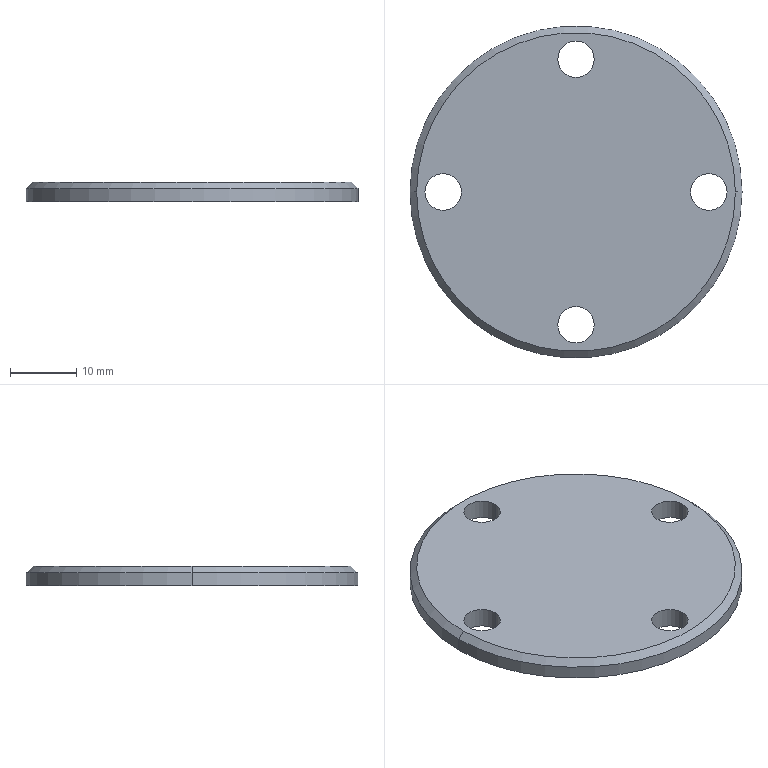Part | SolidWorks | features Chamfer 1, Extrusion 1, ICE 1 | 1 solid | 14 faces | box 50 x 50 x 3 mm | volume 5528 mm3 | cylinder 10 | cone 2 | plane 2 | commonest cylinder face diameters 5.5 x8 50 x2
STEP:
#1=CARTESIAN_POINT('',(17.25,0.,0.));
#2=VERTEX_POINT('',#1);
#3=CARTESIAN_POINT('',(22.75,0.,0.));
#4=VERTEX_POINT('',#3);
#5=CARTESIAN_POINT('',(20.,0.,0.));
#6=DIRECTION('',(0.,0.,1.));
#7=DIRECTION('',(1.,0.,0.));
#8=AXIS2_PLACEMENT_3D('',#5,#6,#7);
#9=CIRCLE('',#8,2.75);
#10=EDGE_CURVE('',#2,#4,#9,.T.);
#11=ORIENTED_EDGE('',*,*,#10,.F.);
#12=CARTESIAN_POINT('',(17.25,0.,3.));
#13=VERTEX_POINT('',#12);
#14=CARTESIAN_POINT('',(17.25,0.,0.));
#15=DIRECTION('',(0.,0.,1.));
#16=VECTOR('',#15,1000.);
#17=LINE('',#14,#16);
#18=EDGE_CURVE('',#2,#13,#17,.T.);
#19=ORIENTED_EDGE('',*,*,#18,.T.);
#20=CARTESIAN_POINT('',(22.75,0.,3.));
#21=VERTEX_POINT('',#20);
#22=CARTESIAN_POINT('',(20.,0.,3.));
#23=DIRECTION('',(0.,0.,1.));
#24=DIRECTION('',(1.,0.,0.));
#25=AXIS2_PLACEMENT_3D('',#22,#23,#24);
#26=CIRCLE('',#25,2.75);
#27=EDGE_CURVE('',#13,#21,#26,.T.);
#28=ORIENTED_EDGE('',*,*,#27,.T.);
#29=CARTESIAN_POINT('',(22.75,0.,0.));
#30=DIRECTION('',(0.,0.,1.));
#31=VECTOR('',#30,1000.);
#32=LINE('',#29,#31);
#33=EDGE_CURVE('',#4,#21,#32,.T.);
#34=ORIENTED_EDGE('',*,*,#33,.F.);
#35=EDGE_LOOP('',(#11,#19,#28,#34));
#36=FACE_OUTER_BOUND('',#35,.T.);
#37=CARTESIAN_POINT('',(20.,0.,0.));
#38=DIRECTION('',(0.,0.,1.));
#39=DIRECTION('',(1.,0.,0.));
#40=AXIS2_PLACEMENT_3D('',#37,#38,#39);
#41=CYLINDRICAL_SURFACE('',#40,2.75);
#42=ADVANCED_FACE('',(#36),#41,.F.);
#43=CARTESIAN_POINT('',(-2.75,-20.,0.));
#44=VERTEX_POINT('',#43);
#45=CARTESIAN_POINT('',(2.75,-20.,0.));
#46=VERTEX_POINT('',#45);
#47=CARTESIAN_POINT('',(0.,-20.,0.));
#48=DIRECTION('',(0.,0.,1.));
#49=DIRECTION('',(1.,0.,0.));
#50=AXIS2_PLACEMENT_3D('',#47,#48,#49);
#51=CIRCLE('',#50,2.75);
#52=EDGE_CURVE('',#44,#46,#51,.T.);
#53=ORIENTED_EDGE('',*,*,#52,.F.);
#54=CARTESIAN_POINT('',(-2.75,-20.,3.));
#55=VERTEX_POINT('',#54);
#56=CARTESIAN_POINT('',(-2.75,-20.,0.));
#57=DIRECTION('',(0.,0.,1.));
#58=VECTOR('',#57,1000.);
#59=LINE('',#56,#58);
#60=EDGE_CURVE('',#44,#55,#59,.T.);
#61=ORIENTED_EDGE('',*,*,#60,.T.);
#62=CARTESIAN_POINT('',(2.75,-20.,3.));
#63=VERTEX_POINT('',#62);
#64=CARTESIAN_POINT('',(0.,-20.,3.));
#65=DIRECTION('',(0.,0.,1.));
#66=DIRECTION('',(1.,0.,0.));
#67=AXIS2_PLACEMENT_3D('',#64,#65,#66);
#68=CIRCLE('',#67,2.75);
#69=EDGE_CURVE('',#55,#63,#68,.T.);
#70=ORIENTED_EDGE('',*,*,#69,.T.);
#71=CARTESIAN_POINT('',(2.75,-20.,0.));
#72=DIRECTION('',(0.,0.,1.));
#73=VECTOR('',#72,1000.);
#74=LINE('',#71,#73);
#75=EDGE_CURVE('',#46,#63,#74,.T.);
#76=ORIENTED_EDGE('',*,*,#75,.F.);
#77=EDGE_LOOP('',(#53,#61,#70,#76));
#78=FACE_OUTER_BOUND('',#77,.T.);
#79=CARTESIAN_POINT('',(0.,-20.,0.));
#80=DIRECTION('',(0.,0.,1.));
#81=DIRECTION('',(1.,0.,0.));
#82=AXIS2_PLACEMENT_3D('',#79,#80,#81);
#83=CYLINDRICAL_SURFACE('',#82,2.75);
#84=ADVANCED_FACE('',(#78),#83,.F.);
#85=CARTESIAN_POINT('',(-22.75,0.,0.));
#86=VERTEX_POINT('',#85);
#87=CARTESIAN_POINT('',(-17.25,0.,0.));
#88=VERTEX_POINT('',#87);
#89=CARTESIAN_POINT('',(-20.,0.,0.));
#90=DIRECTION('',(0.,0.,1.));
#91=DIRECTION('',(1.,0.,0.));
#92=AXIS2_PLACEMENT_3D('',#89,#90,#91);
#93=CIRCLE('',#92,2.75);
#94=EDGE_CURVE('',#86,#88,#93,.T.);
#95=ORIENTED_EDGE('',*,*,#94,.F.);
#96=CARTESIAN_POINT('',(-22.75,0.,3.));
#97=VERTEX_POINT('',#96);
#98=CARTESIAN_POINT('',(-22.75,0.,0.));
#99=DIRECTION('',(0.,0.,1.));
#100=VECTOR('',#99,1000.);
#101=LINE('',#98,#100);
#102=EDGE_CURVE('',#86,#97,#101,.T.);
#103=ORIENTED_EDGE('',*,*,#102,.T.);
#104=CARTESIAN_POINT('',(-17.25,0.,3.));
#105=VERTEX_POINT('',#104);
#106=CARTESIAN_POINT('',(-20.,0.,3.));
#107=DIRECTION('',(0.,0.,1.));
#108=DIRECTION('',(1.,0.,0.));
#109=AXIS2_PLACEMENT_3D('',#106,#107,#108);
#110=CIRCLE('',#109,2.75);
#111=EDGE_CURVE('',#97,#105,#110,.T.);
#112=ORIENTED_EDGE('',*,*,#111,.T.);
#113=CARTESIAN_POINT('',(-17.25,0.,0.));
#114=DIRECTION('',(0.,0.,1.));
#115=VECTOR('',#114,1000.);
#116=LINE('',#113,#115);
#117=EDGE_CURVE('',#88,#105,#116,.T.);
#118=ORIENTED_EDGE('',*,*,#117,.F.);
#119=EDGE_LOOP('',(#95,#103,#112,#118));
#120=FACE_OUTER_BOUND('',#119,.T.);
#121=CARTESIAN_POINT('',(-20.,0.,0.));
#122=DIRECTION('',(0.,0.,1.));
#123=DIRECTION('',(1.,0.,0.));
#124=AXIS2_PLACEMENT_3D('',#121,#122,#123);
#125=CYLINDRICAL_SURFACE('',#124,2.75);
#126=ADVANCED_FACE('',(#120),#125,.F.);
#127=CARTESIAN_POINT('',(-2.75,20.,0.));
#128=VERTEX_POINT('',#127);
#129=CARTESIAN_POINT('',(2.75,20.,0.));
#130=VERTEX_POINT('',#129);
#131=CARTESIAN_POINT('',(0.,20.,0.));
#132=DIRECTION('',(0.,0.,1.));
#133=DIRECTION('',(1.,0.,0.));
#134=AXIS2_PLACEMENT_3D('',#131,#132,#133);
#135=CIRCLE('',#134,2.75);
#136=EDGE_CURVE('',#128,#130,#135,.T.);
#137=ORIENTED_EDGE('',*,*,#136,.F.);
#138=CARTESIAN_POINT('',(-2.75,20.,3.));
#139=VERTEX_POINT('',#138);
#140=CARTESIAN_POINT('',(-2.75,20.,0.));
#141=DIRECTION('',(0.,0.,1.));
#142=VECTOR('',#141,1000.);
#143=LINE('',#140,#142);
#144=EDGE_CURVE('',#128,#139,#143,.T.);
#145=ORIENTED_EDGE('',*,*,#144,.T.);
#146=CARTESIAN_POINT('',(2.75,20.,3.));
#147=VERTEX_POINT('',#146);
#148=CARTESIAN_POINT('',(0.,20.,3.));
#149=DIRECTION('',(0.,0.,1.));
#150=DIRECTION('',(1.,0.,0.));
#151=AXIS2_PLACEMENT_3D('',#148,#149,#150);
#152=CIRCLE('',#151,2.75);
#153=EDGE_CURVE('',#139,#147,#152,.T.);
#154=ORIENTED_EDGE('',*,*,#153,.T.);
#155=CARTESIAN_POINT('',(2.75,20.,0.));
#156=DIRECTION('',(0.,0.,1.));
#157=VECTOR('',#156,1000.);
#158=LINE('',#155,#157);
#159=EDGE_CURVE('',#130,#147,#158,.T.);
#160=ORIENTED_EDGE('',*,*,#159,.F.);
#161=EDGE_LOOP('',(#137,#145,#154,#160));
#162=FACE_OUTER_BOUND('',#161,.T.);
#163=CARTESIAN_POINT('',(0.,20.,0.));
#164=DIRECTION('',(0.,0.,1.));
#165=DIRECTION('',(1.,0.,0.));
#166=AXIS2_PLACEMENT_3D('',#163,#164,#165);
#167=CYLINDRICAL_SURFACE('',#166,2.75);
#168=ADVANCED_FACE('',(#162),#167,.F.);
#169=CARTESIAN_POINT('',(24.,0.,3.));
#170=VERTEX_POINT('',#169);
#171=CARTESIAN_POINT('',(-24.,0.,3.));
#172=VERTEX_POINT('',#171);
#173=CARTESIAN_POINT('',(0.,0.,3.));
#174=DIRECTION('',(0.,0.,1.));
#175=DIRECTION('',(1.,0.,0.));
#176=AXIS2_PLACEMENT_3D('',#173,#174,#175);
#177=CIRCLE('',#176,24.);
#178=EDGE_CURVE('',#170,#172,#177,.T.);
#179=ORIENTED_EDGE('',*,*,#178,.F.);
#180=CARTESIAN_POINT('',(25.,0.,2.));
#181=VERTEX_POINT('',#180);
#182=CARTESIAN_POINT('',(24.,0.,3.));
#183=DIRECTION('',(0.7071,0.,-0.7071));
#184=VECTOR('',#183,1000.);
#185=LINE('',#182,#184);
#186=EDGE_CURVE('',#170,#181,#185,.T.);
#187=ORIENTED_EDGE('',*,*,#186,.T.);
#188=CARTESIAN_POINT('',(-25.,0.,2.));
#189=VERTEX_POINT('',#188);
#190=CARTESIAN_POINT('',(0.,0.,2.));
#191=DIRECTION('',(0.,0.,-1.));
#192=DIRECTION('',(1.,0.,0.));
#193=AXIS2_PLACEMENT_3D('',#190,#191,#192);
#194=CIRCLE('',#193,25.);
#195=EDGE_CURVE('',#189,#181,#194,.T.);
#196=ORIENTED_EDGE('',*,*,#195,.F.);
#197=CARTESIAN_POINT('',(-24.,0.,3.));
#198=DIRECTION('',(-0.7071,0.,-0.7071));
#199=VECTOR('',#198,1000.);
#200=LINE('',#197,#199);
#201=EDGE_CURVE('',#172,#189,#200,.T.);
#202=ORIENTED_EDGE('',*,*,#201,.F.);
#203=EDGE_LOOP('',(#179,#187,#196,#202));
#204=FACE_OUTER_BOUND('',#203,.T.);
#205=CARTESIAN_POINT('',(0.,0.,3.));
#206=DIRECTION('',(0.,0.,-1.));
#207=DIRECTION('',(-1.,0.,0.));
#208=AXIS2_PLACEMENT_3D('',#205,#206,#207);
#209=CONICAL_SURFACE('',#208,24.,0.7854);
#210=ADVANCED_FACE('',(#204),#209,.T.);
#211=ORIENTED_EDGE('',*,*,#195,.T.);
#212=CARTESIAN_POINT('',(25.,0.,0.));
#213=VERTEX_POINT('',#212);
#214=CARTESIAN_POINT('',(25.,0.,3.));
#215=DIRECTION('',(0.,0.,-1.));
#216=VECTOR('',#215,1000.);
#217=LINE('',#214,#216);
#218=EDGE_CURVE('',#181,#213,#217,.T.);
#219=ORIENTED_EDGE('',*,*,#218,.T.);
#220=CARTESIAN_POINT('',(-25.,0.,0.));
#221=VERTEX_POINT('',#220);
#222=CARTESIAN_POINT('',(0.,0.,0.));
#223=DIRECTION('',(0.,0.,1.));
#224=DIRECTION('',(1.,0.,0.));
#225=AXIS2_PLACEMENT_3D('',#222,#223,#224);
#226=CIRCLE('',#225,25.);
#227=EDGE_CURVE('',#213,#221,#226,.T.);
#228=ORIENTED_EDGE('',*,*,#227,.T.);
#229=CARTESIAN_POINT('',(-25.,0.,3.));
#230=DIRECTION('',(0.,0.,-1.));
#231=VECTOR('',#230,1000.);
#232=LINE('',#229,#231);
#233=EDGE_CURVE('',#189,#221,#232,.T.);
#234=ORIENTED_EDGE('',*,*,#233,.F.);
#235=EDGE_LOOP('',(#211,#219,#228,#234));
#236=FACE_OUTER_BOUND('',#235,.T.);
#237=CARTESIAN_POINT('',(0.,0.,3.));
#238=DIRECTION('',(0.,0.,-1.));
#239=DIRECTION('',(-1.,0.,0.));
#240=AXIS2_PLACEMENT_3D('',#237,#238,#239);
#241=CYLINDRICAL_SURFACE('',#240,25.);
#242=ADVANCED_FACE('',(#236),#241,.T.);
#243=ORIENTED_EDGE('',*,*,#218,.F.);
#244=CARTESIAN_POINT('',(0.,0.,2.));
#245=DIRECTION('',(0.,0.,-1.));
#246=DIRECTION('',(1.,0.,0.));
#247=AXIS2_PLACEMENT_3D('',#244,#245,#246);
#248=CIRCLE('',#247,25.);
#249=EDGE_CURVE('',#181,#189,#248,.T.);
#250=ORIENTED_EDGE('',*,*,#249,.T.);
#251=ORIENTED_EDGE('',*,*,#233,.T.);
#252=CARTESIAN_POINT('',(0.,0.,0.));
#253=DIRECTION('',(0.,0.,1.));
#254=DIRECTION('',(1.,0.,0.));
#255=AXIS2_PLACEMENT_3D('',#252,#253,#254);
#256=CIRCLE('',#255,25.);
#257=EDGE_CURVE('',#221,#213,#256,.T.);
#258=ORIENTED_EDGE('',*,*,#257,.T.);
#259=EDGE_LOOP('',(#243,#250,#251,#258));
#260=FACE_OUTER_BOUND('',#259,.T.);
#261=CARTESIAN_POINT('',(0.,0.,3.));
#262=DIRECTION('',(0.,0.,-1.));
#263=DIRECTION('',(-1.,0.,0.));
#264=AXIS2_PLACEMENT_3D('',#261,#262,#263);
#265=CYLINDRICAL_SURFACE('',#264,25.);
#266=ADVANCED_FACE('',(#260),#265,.T.);
#267=CARTESIAN_POINT('',(20.,0.,3.));
#268=DIRECTION('',(0.,0.,1.));
#269=DIRECTION('',(1.,0.,0.));
#270=AXIS2_PLACEMENT_3D('',#267,#268,#269);
#271=CIRCLE('',#270,2.75);
#272=EDGE_CURVE('',#21,#13,#271,.T.);
#273=ORIENTED_EDGE('',*,*,#272,.F.);
#274=ORIENTED_EDGE('',*,*,#27,.F.);
#275=EDGE_LOOP('',(#273,#274));
#276=FACE_BOUND('',#275,.T.);
#277=CARTESIAN_POINT('',(0.,-20.,3.));
#278=DIRECTION('',(0.,0.,1.));
#279=DIRECTION('',(1.,0.,0.));
#280=AXIS2_PLACEMENT_3D('',#277,#278,#279);
#281=CIRCLE('',#280,2.75);
#282=EDGE_CURVE('',#63,#55,#281,.T.);
#283=ORIENTED_EDGE('',*,*,#282,.F.);
#284=ORIENTED_EDGE('',*,*,#69,.F.);
#285=EDGE_LOOP('',(#283,#284));
#286=FACE_BOUND('',#285,.T.);
#287=CARTESIAN_POINT('',(-20.,0.,3.));
#288=DIRECTION('',(0.,0.,1.));
#289=DIRECTION('',(1.,0.,0.));
#290=AXIS2_PLACEMENT_3D('',#287,#288,#289);
#291=CIRCLE('',#290,2.75);
#292=EDGE_CURVE('',#105,#97,#291,.T.);
#293=ORIENTED_EDGE('',*,*,#292,.F.);
#294=ORIENTED_EDGE('',*,*,#111,.F.);
#295=EDGE_LOOP('',(#293,#294));
#296=FACE_BOUND('',#295,.T.);
#297=CARTESIAN_POINT('',(0.,20.,3.));
#298=DIRECTION('',(0.,0.,1.));
#299=DIRECTION('',(1.,0.,0.));
#300=AXIS2_PLACEMENT_3D('',#297,#298,#299);
#301=CIRCLE('',#300,2.75);
#302=EDGE_CURVE('',#147,#139,#301,.T.);
#303=ORIENTED_EDGE('',*,*,#302,.F.);
#304=ORIENTED_EDGE('',*,*,#153,.F.);
#305=EDGE_LOOP('',(#303,#304));
#306=FACE_BOUND('',#305,.T.);
#307=CARTESIAN_POINT('',(0.,0.,3.));
#308=DIRECTION('',(0.,0.,1.));
#309=DIRECTION('',(1.,0.,0.));
#310=AXIS2_PLACEMENT_3D('',#307,#308,#309);
#311=CIRCLE('',#310,24.);
#312=EDGE_CURVE('',#172,#170,#311,.T.);
#313=ORIENTED_EDGE('',*,*,#312,.T.);
#314=ORIENTED_EDGE('',*,*,#178,.T.);
#315=EDGE_LOOP('',(#313,#314));
#316=FACE_OUTER_BOUND('',#315,.T.);
#317=CARTESIAN_POINT('',(0.,0.,3.));
#318=DIRECTION('',(0.,0.,1.));
#319=DIRECTION('',(1.,0.,0.));
#320=AXIS2_PLACEMENT_3D('',#317,#318,#319);
#321=PLANE('',#320);
#322=ADVANCED_FACE('',(#276,#286,#296,#306,#316),#321,.T.);
#323=CARTESIAN_POINT('',(20.,0.,0.));
#324=DIRECTION('',(0.,0.,1.));
#325=DIRECTION('',(1.,0.,0.));
#326=AXIS2_PLACEMENT_3D('',#323,#324,#325);
#327=CIRCLE('',#326,2.75);
#328=EDGE_CURVE('',#4,#2,#327,.T.);
#329=ORIENTED_EDGE('',*,*,#328,.T.);
#330=ORIENTED_EDGE('',*,*,#10,.T.);
#331=EDGE_LOOP('',(#329,#330));
#332=FACE_BOUND('',#331,.T.);
#333=CARTESIAN_POINT('',(0.,-20.,0.));
#334=DIRECTION('',(0.,0.,1.));
#335=DIRECTION('',(1.,0.,0.));
#336=AXIS2_PLACEMENT_3D('',#333,#334,#335);
#337=CIRCLE('',#336,2.75);
#338=EDGE_CURVE('',#46,#44,#337,.T.);
#339=ORIENTED_EDGE('',*,*,#338,.T.);
#340=ORIENTED_EDGE('',*,*,#52,.T.);
#341=EDGE_LOOP('',(#339,#340));
#342=FACE_BOUND('',#341,.T.);
#343=CARTESIAN_POINT('',(-20.,0.,0.));
#344=DIRECTION('',(0.,0.,1.));
#345=DIRECTION('',(1.,0.,0.));
#346=AXIS2_PLACEMENT_3D('',#343,#344,#345);
#347=CIRCLE('',#346,2.75);
#348=EDGE_CURVE('',#88,#86,#347,.T.);
#349=ORIENTED_EDGE('',*,*,#348,.T.);
#350=ORIENTED_EDGE('',*,*,#94,.T.);
#351=EDGE_LOOP('',(#349,#350));
#352=FACE_BOUND('',#351,.T.);
#353=CARTESIAN_POINT('',(0.,20.,0.));
#354=DIRECTION('',(0.,0.,1.));
#355=DIRECTION('',(1.,0.,0.));
#356=AXIS2_PLACEMENT_3D('',#353,#354,#355);
#357=CIRCLE('',#356,2.75);
#358=EDGE_CURVE('',#130,#128,#357,.T.);
#359=ORIENTED_EDGE('',*,*,#358,.T.);
#360=ORIENTED_EDGE('',*,*,#136,.T.);
#361=EDGE_LOOP('',(#359,#360));
#362=FACE_BOUND('',#361,.T.);
#363=ORIENTED_EDGE('',*,*,#257,.F.);
#364=ORIENTED_EDGE('',*,*,#227,.F.);
#365=EDGE_LOOP('',(#363,#364));
#366=FACE_OUTER_BOUND('',#365,.T.);
#367=CARTESIAN_POINT('',(0.,0.,0.));
#368=DIRECTION('',(0.,0.,1.));
#369=DIRECTION('',(1.,0.,0.));
#370=AXIS2_PLACEMENT_3D('',#367,#368,#369);
#371=PLANE('',#370);
#372=ADVANCED_FACE('',(#332,#342,#352,#362,#366),#371,.F.);
#373=ORIENTED_EDGE('',*,*,#186,.F.);
#374=ORIENTED_EDGE('',*,*,#312,.F.);
#375=ORIENTED_EDGE('',*,*,#201,.T.);
#376=ORIENTED_EDGE('',*,*,#249,.F.);
#377=EDGE_LOOP('',(#373,#374,#375,#376));
#378=FACE_OUTER_BOUND('',#377,.T.);
#379=CARTESIAN_POINT('',(0.,0.,3.));
#380=DIRECTION('',(0.,0.,-1.));
#381=DIRECTION('',(-1.,0.,0.));
#382=AXIS2_PLACEMENT_3D('',#379,#380,#381);
#383=CONICAL_SURFACE('',#382,24.,0.7854);
#384=ADVANCED_FACE('',(#378),#383,.T.);
#385=ORIENTED_EDGE('',*,*,#144,.F.);
#386=ORIENTED_EDGE('',*,*,#358,.F.);
#387=ORIENTED_EDGE('',*,*,#159,.T.);
#388=ORIENTED_EDGE('',*,*,#302,.T.);
#389=EDGE_LOOP('',(#385,#386,#387,#388));
#390=FACE_OUTER_BOUND('',#389,.T.);
#391=CARTESIAN_POINT('',(0.,20.,0.));
#392=DIRECTION('',(0.,0.,1.));
#393=DIRECTION('',(1.,0.,0.));
#394=AXIS2_PLACEMENT_3D('',#391,#392,#393);
#395=CYLINDRICAL_SURFACE('',#394,2.75);
#396=ADVANCED_FACE('',(#390),#395,.F.);
#397=ORIENTED_EDGE('',*,*,#102,.F.);
#398=ORIENTED_EDGE('',*,*,#348,.F.);
#399=ORIENTED_EDGE('',*,*,#117,.T.);
#400=ORIENTED_EDGE('',*,*,#292,.T.);
#401=EDGE_LOOP('',(#397,#398,#399,#400));
#402=FACE_OUTER_BOUND('',#401,.T.);
#403=CARTESIAN_POINT('',(-20.,0.,0.));
#404=DIRECTION('',(0.,0.,1.));
#405=DIRECTION('',(1.,0.,0.));
#406=AXIS2_PLACEMENT_3D('',#403,#404,#405);
#407=CYLINDRICAL_SURFACE('',#406,2.75);
#408=ADVANCED_FACE('',(#402),#407,.F.);
#409=ORIENTED_EDGE('',*,*,#60,.F.);
#410=ORIENTED_EDGE('',*,*,#338,.F.);
#411=ORIENTED_EDGE('',*,*,#75,.T.);
#412=ORIENTED_EDGE('',*,*,#282,.T.);
#413=EDGE_LOOP('',(#409,#410,#411,#412));
#414=FACE_OUTER_BOUND('',#413,.T.);
#415=CARTESIAN_POINT('',(0.,-20.,0.));
#416=DIRECTION('',(0.,0.,1.));
#417=DIRECTION('',(1.,0.,0.));
#418=AXIS2_PLACEMENT_3D('',#415,#416,#417);
#419=CYLINDRICAL_SURFACE('',#418,2.75);
#420=ADVANCED_FACE('',(#414),#419,.F.);
#421=ORIENTED_EDGE('',*,*,#18,.F.);
#422=ORIENTED_EDGE('',*,*,#328,.F.);
#423=ORIENTED_EDGE('',*,*,#33,.T.);
#424=ORIENTED_EDGE('',*,*,#272,.T.);
#425=EDGE_LOOP('',(#421,#422,#423,#424));
#426=FACE_OUTER_BOUND('',#425,.T.);
#427=CARTESIAN_POINT('',(20.,0.,0.));
#428=DIRECTION('',(0.,0.,1.));
#429=DIRECTION('',(1.,0.,0.));
#430=AXIS2_PLACEMENT_3D('',#427,#428,#429);
#431=CYLINDRICAL_SURFACE('',#430,2.75);
#432=ADVANCED_FACE('',(#426),#431,.F.);
#433=CLOSED_SHELL('',(#42,#84,#126,#168,#210,#242,#266,#322,#372,#384,#396,#408,#420,#432));
#434=MANIFOLD_SOLID_BREP('',#433);
#435=CARTESIAN_POINT('',(0.,0.,0.));
#436=DIRECTION('',(0.,0.,1.));
#437=DIRECTION('',(1.,0.,0.));
#438=AXIS2_PLACEMENT_3D('',#435,#436,#437);
#439=(LENGTH_UNIT()NAMED_UNIT(*)SI_UNIT(.MILLI.,.METRE.));
#440=UNCERTAINTY_MEASURE_WITH_UNIT(LENGTH_MEASURE(0.00001),#439,'','');
#441=(NAMED_UNIT(*)PLANE_ANGLE_UNIT()SI_UNIT($,.RADIAN.));
#442=(NAMED_UNIT(*)SI_UNIT($,.STERADIAN.)SOLID_ANGLE_UNIT());
#443=(GEOMETRIC_REPRESENTATION_CONTEXT(3)GLOBAL_UNCERTAINTY_ASSIGNED_CONTEXT((#440))GLOBAL_UNIT_ASSIGNED_CONTEXT((#439,#441,#442))REPRESENTATION_CONTEXT('',''));
#444=ADVANCED_BREP_SHAPE_REPRESENTATION('',(#434,#438),#443);